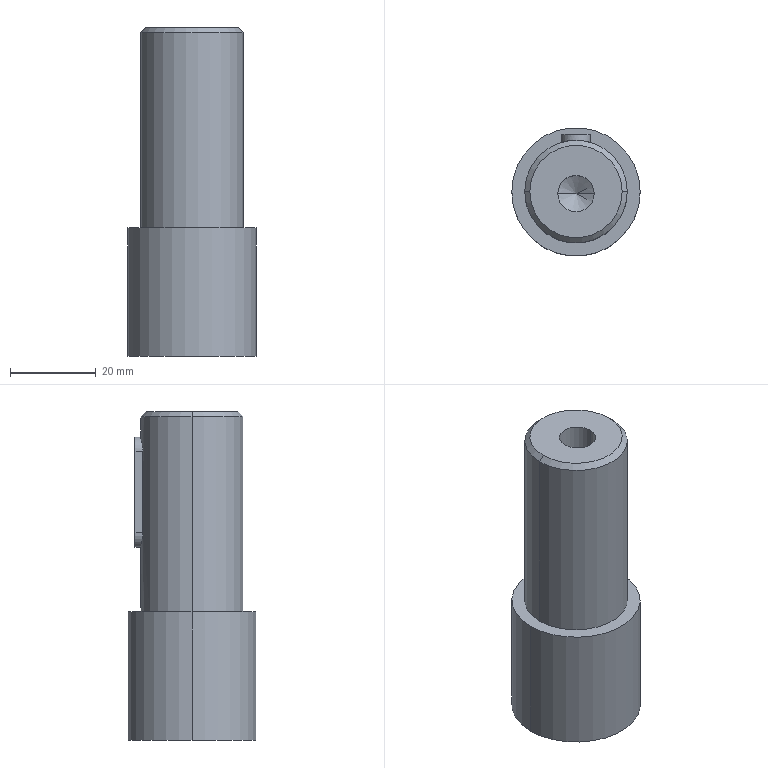Part | STEP file | XB output shaft_100_165_28.step | 1 solid | 24 faces | box 30 x 30 x 76.8 mm | volume 41146 mm3 | cylinder 9 | plane 8 | cone 7 | commonest cylinder face diameters 6.72 x3 8.5 x2 24 x2 30 x2
STEP:
#1=CARTESIAN_POINT('',(-4.25,0.,-98.603));
#2=VERTEX_POINT('',#1);
#3=CARTESIAN_POINT('',(4.25,0.,-98.603));
#4=VERTEX_POINT('',#3);
#5=CARTESIAN_POINT('',(0.,0.,-98.603));
#6=DIRECTION('',(0.,0.,1.));
#7=DIRECTION('',(1.,0.,0.));
#8=AXIS2_PLACEMENT_3D('',#5,#6,#7);
#9=CIRCLE('',#8,4.25);
#10=EDGE_CURVE('',#2,#4,#9,.T.);
#11=ORIENTED_EDGE('',*,*,#10,.F.);
#12=CARTESIAN_POINT('',(-4.25,0.,-74.103));
#13=VERTEX_POINT('',#12);
#14=CARTESIAN_POINT('',(-4.25,0.,-74.103));
#15=DIRECTION('',(0.,0.,1.));
#16=VECTOR('',#15,1000.);
#17=LINE('',#14,#16);
#18=EDGE_CURVE('',#2,#13,#17,.T.);
#19=ORIENTED_EDGE('',*,*,#18,.T.);
#20=CARTESIAN_POINT('',(4.25,0.,-74.103));
#21=VERTEX_POINT('',#20);
#22=CARTESIAN_POINT('',(0.,0.,-74.103));
#23=DIRECTION('',(0.,0.,1.));
#24=DIRECTION('',(1.,0.,0.));
#25=AXIS2_PLACEMENT_3D('',#22,#23,#24);
#26=CIRCLE('',#25,4.25);
#27=EDGE_CURVE('',#13,#21,#26,.T.);
#28=ORIENTED_EDGE('',*,*,#27,.T.);
#29=CARTESIAN_POINT('',(4.25,0.,-74.103));
#30=DIRECTION('',(0.,0.,1.));
#31=VECTOR('',#30,1000.);
#32=LINE('',#29,#31);
#33=EDGE_CURVE('',#4,#21,#32,.T.);
#34=ORIENTED_EDGE('',*,*,#33,.F.);
#35=EDGE_LOOP('',(#11,#19,#28,#34));
#36=FACE_OUTER_BOUND('',#35,.T.);
#37=CARTESIAN_POINT('',(0.,0.,-74.103));
#38=DIRECTION('',(0.,0.,1.));
#39=DIRECTION('',(1.,0.,0.));
#40=AXIS2_PLACEMENT_3D('',#37,#38,#39);
#41=CYLINDRICAL_SURFACE('',#40,4.25);
#42=ADVANCED_FACE('',(#36),#41,.F.);
#43=CARTESIAN_POINT('',(0.,0.,-101.156));
#44=VERTEX_POINT('',#43);
#45=CARTESIAN_POINT('',(4.25,0.,-98.603));
#46=DIRECTION('',(0.8572,0.,0.515));
#47=VECTOR('',#46,1000.);
#48=LINE('',#45,#47);
#49=EDGE_CURVE('',#44,#4,#48,.T.);
#50=ORIENTED_EDGE('',*,*,#49,.F.);
#51=CARTESIAN_POINT('',(-4.25,0.,-98.603));
#52=DIRECTION('',(-0.8572,0.,0.515));
#53=VECTOR('',#52,1000.);
#54=LINE('',#51,#53);
#55=EDGE_CURVE('',#44,#2,#54,.T.);
#56=ORIENTED_EDGE('',*,*,#55,.T.);
#57=ORIENTED_EDGE('',*,*,#10,.T.);
#58=EDGE_LOOP('',(#50,#56,#57));
#59=FACE_OUTER_BOUND('',#58,.T.);
#60=CARTESIAN_POINT('',(0.,0.,-98.603));
#61=DIRECTION('',(0.,0.,1.));
#62=DIRECTION('',(1.,0.,0.));
#63=AXIS2_PLACEMENT_3D('',#60,#61,#62);
#64=CONICAL_SURFACE('',#63,4.25,1.03);
#65=ADVANCED_FACE('',(#59),#64,.F.);
#66=CARTESIAN_POINT('',(-15.,0.4853,-150.903));
#67=VERTEX_POINT('',#66);
#68=CARTESIAN_POINT('',(15.,0.4853,-150.903));
#69=VERTEX_POINT('',#68);
#70=CARTESIAN_POINT('',(0.000002753,0.4853,-150.903));
#71=DIRECTION('',(0.,0.,-1.));
#72=DIRECTION('',(-1.,0.,0.));
#73=AXIS2_PLACEMENT_3D('',#70,#71,#72);
#74=CIRCLE('',#73,15.);
#75=EDGE_CURVE('',#67,#69,#74,.T.);
#76=ORIENTED_EDGE('',*,*,#75,.F.);
#77=CARTESIAN_POINT('',(-15.,0.4853,-120.903));
#78=VERTEX_POINT('',#77);
#79=CARTESIAN_POINT('',(-15.,0.4853,-150.903));
#80=DIRECTION('',(0.,0.,1.));
#81=VECTOR('',#80,1000.);
#82=LINE('',#79,#81);
#83=EDGE_CURVE('',#67,#78,#82,.T.);
#84=ORIENTED_EDGE('',*,*,#83,.T.);
#85=CARTESIAN_POINT('',(15.,0.4853,-120.903));
#86=VERTEX_POINT('',#85);
#87=CARTESIAN_POINT('',(0.000002753,0.4853,-120.903));
#88=DIRECTION('',(0.,0.,-1.));
#89=DIRECTION('',(-1.,0.,0.));
#90=AXIS2_PLACEMENT_3D('',#87,#88,#89);
#91=CIRCLE('',#90,15.);
#92=EDGE_CURVE('',#78,#86,#91,.T.);
#93=ORIENTED_EDGE('',*,*,#92,.T.);
#94=CARTESIAN_POINT('',(15.,0.4853,-150.903));
#95=DIRECTION('',(0.,0.,1.));
#96=VECTOR('',#95,1000.);
#97=LINE('',#94,#96);
#98=EDGE_CURVE('',#69,#86,#97,.T.);
#99=ORIENTED_EDGE('',*,*,#98,.F.);
#100=EDGE_LOOP('',(#76,#84,#93,#99));
#101=FACE_OUTER_BOUND('',#100,.T.);
#102=CARTESIAN_POINT('',(0.000002753,0.4853,-150.903));
#103=DIRECTION('',(0.,0.,1.));
#104=DIRECTION('',(1.,0.,0.));
#105=AXIS2_PLACEMENT_3D('',#102,#103,#104);
#106=CYLINDRICAL_SURFACE('',#105,15.);
#107=ADVANCED_FACE('',(#101),#106,.T.);
#108=CARTESIAN_POINT('',(-3.36,12.005,-83.403));
#109=VERTEX_POINT('',#108);
#110=CARTESIAN_POINT('',(-3.36,12.005,-102.423));
#111=VERTEX_POINT('',#110);
#112=CARTESIAN_POINT('',(-3.36,12.005,-74.103));
#113=DIRECTION('',(0.,0.,-1.));
#114=VECTOR('',#113,1000.);
#115=LINE('',#112,#114);
#116=EDGE_CURVE('',#109,#111,#115,.T.);
#117=ORIENTED_EDGE('',*,*,#116,.T.);
#118=CARTESIAN_POINT('',(0.000002753,12.485,-105.783));
#119=VERTEX_POINT('',#118);
#120=CARTESIAN_POINT('',(-3.36,12.005,-102.423));
#121=CARTESIAN_POINT('',(-3.36,12.005,-102.646));
#122=CARTESIAN_POINT('',(-3.338,12.012,-102.865));
#123=CARTESIAN_POINT('',(-3.252,12.036,-103.295));
#124=CARTESIAN_POINT('',(-3.187,12.055,-103.509));
#125=CARTESIAN_POINT('',(-3.018,12.1,-103.915));
#126=CARTESIAN_POINT('',(-2.915,12.127,-104.108));
#127=CARTESIAN_POINT('',(-2.672,12.185,-104.472));
#128=CARTESIAN_POINT('',(-2.531,12.216,-104.644));
#129=CARTESIAN_POINT('',(-2.223,12.279,-104.952));
#130=CARTESIAN_POINT('',(-2.054,12.31,-105.09));
#131=CARTESIAN_POINT('',(-1.688,12.367,-105.336));
#132=CARTESIAN_POINT('',(-1.494,12.394,-105.44));
#133=CARTESIAN_POINT('',(-1.091,12.437,-105.608));
#134=CARTESIAN_POINT('',(-0.8782,12.455,-105.673));
#135=CARTESIAN_POINT('',(-0.4433,12.479,-105.761));
#136=CARTESIAN_POINT('',(-0.223,12.485,-105.783));
#137=CARTESIAN_POINT('',(0.000002753,12.485,-105.783));
#138=B_SPLINE_CURVE_WITH_KNOTS('',3,(#120,#121,#122,#123,#124,#125,#126,#127,#128,#129,#130,#131,#132,#133,#134,#135,#136,#137),.UNSPECIFIED.,.F.,.F.,(4,2,2,2,2,2,2,2,4),(0.,0.0006594,0.001319,0.001978,0.002638,0.003297,0.003957,0.004616,0.005275),.UNSPECIFIED.);
#139=EDGE_CURVE('',#111,#119,#138,.T.);
#140=ORIENTED_EDGE('',*,*,#139,.T.);
#141=CARTESIAN_POINT('',(3.36,12.005,-102.423));
#142=VERTEX_POINT('',#141);
#143=CARTESIAN_POINT('',(0.000002753,12.485,-105.783));
#144=CARTESIAN_POINT('',(0.2231,12.485,-105.783));
#145=CARTESIAN_POINT('',(0.4422,12.479,-105.761));
#146=CARTESIAN_POINT('',(0.8729,12.455,-105.675));
#147=CARTESIAN_POINT('',(1.087,12.438,-105.609));
#148=CARTESIAN_POINT('',(1.493,12.394,-105.441));
#149=CARTESIAN_POINT('',(1.686,12.368,-105.337));
#150=CARTESIAN_POINT('',(2.05,12.31,-105.094));
#151=CARTESIAN_POINT('',(2.221,12.279,-104.953));
#152=CARTESIAN_POINT('',(2.53,12.217,-104.645));
#153=CARTESIAN_POINT('',(2.668,12.186,-104.477));
#154=CARTESIAN_POINT('',(2.914,12.127,-104.11));
#155=CARTESIAN_POINT('',(3.018,12.1,-103.916));
#156=CARTESIAN_POINT('',(3.186,12.055,-103.513));
#157=CARTESIAN_POINT('',(3.251,12.037,-103.301));
#158=CARTESIAN_POINT('',(3.338,12.012,-102.866));
#159=CARTESIAN_POINT('',(3.36,12.005,-102.646));
#160=CARTESIAN_POINT('',(3.36,12.005,-102.423));
#161=B_SPLINE_CURVE_WITH_KNOTS('',3,(#143,#144,#145,#146,#147,#148,#149,#150,#151,#152,#153,#154,#155,#156,#157,#158,#159,#160),.UNSPECIFIED.,.F.,.F.,(4,2,2,2,2,2,2,2,4),(0.005275,0.005935,0.006594,0.007254,0.007913,0.008573,0.009232,0.009891,0.01055),.UNSPECIFIED.);
#162=EDGE_CURVE('',#119,#142,#161,.T.);
#163=ORIENTED_EDGE('',*,*,#162,.T.);
#164=CARTESIAN_POINT('',(3.36,12.005,-83.403));
#165=VERTEX_POINT('',#164);
#166=CARTESIAN_POINT('',(3.36,12.005,-74.103));
#167=DIRECTION('',(0.,0.,1.));
#168=VECTOR('',#167,1000.);
#169=LINE('',#166,#168);
#170=EDGE_CURVE('',#142,#165,#169,.T.);
#171=ORIENTED_EDGE('',*,*,#170,.T.);
#172=CARTESIAN_POINT('',(3.36,12.005,-83.403));
#173=CARTESIAN_POINT('',(3.36,12.005,-83.179));
#174=CARTESIAN_POINT('',(3.338,12.012,-82.96));
#175=CARTESIAN_POINT('',(3.252,12.036,-82.529));
#176=CARTESIAN_POINT('',(3.187,12.055,-82.315));
#177=CARTESIAN_POINT('',(3.018,12.1,-81.909));
#178=CARTESIAN_POINT('',(2.915,12.127,-81.717));
#179=CARTESIAN_POINT('',(2.671,12.185,-81.352));
#180=CARTESIAN_POINT('',(2.53,12.217,-81.181));
#181=CARTESIAN_POINT('',(2.222,12.279,-80.873));
#182=CARTESIAN_POINT('',(2.054,12.31,-80.734));
#183=CARTESIAN_POINT('',(1.687,12.368,-80.488));
#184=CARTESIAN_POINT('',(1.493,12.394,-80.385));
#185=CARTESIAN_POINT('',(1.089,12.437,-80.216));
#186=CARTESIAN_POINT('',(0.8764,12.455,-80.151));
#187=CARTESIAN_POINT('',(0.4422,12.479,-80.064));
#188=CARTESIAN_POINT('',(0.2235,12.485,-80.043));
#189=CARTESIAN_POINT('',(-0.2172,12.485,-80.042));
#190=CARTESIAN_POINT('',(-0.441,12.479,-80.064));
#191=CARTESIAN_POINT('',(-0.8729,12.455,-80.15));
#192=CARTESIAN_POINT('',(-1.083,12.438,-80.214));
#193=CARTESIAN_POINT('',(-1.695,12.372,-80.468));
#194=CARTESIAN_POINT('',(-2.064,12.311,-80.715));
#195=CARTESIAN_POINT('',(-2.53,12.217,-81.181));
#196=CARTESIAN_POINT('',(-2.669,12.185,-81.349));
#197=CARTESIAN_POINT('',(-2.912,12.127,-81.712));
#198=CARTESIAN_POINT('',(-3.018,12.1,-81.909));
#199=CARTESIAN_POINT('',(-3.186,12.055,-82.314));
#200=CARTESIAN_POINT('',(-3.25,12.037,-82.523));
#201=CARTESIAN_POINT('',(-3.338,12.012,-82.956));
#202=CARTESIAN_POINT('',(-3.36,12.005,-83.179));
#203=CARTESIAN_POINT('',(-3.36,12.005,-83.403));
#204=B_SPLINE_CURVE_WITH_KNOTS('',3,(#172,#173,#174,#175,#176,#177,#178,#179,#180,#181,#182,#183,#184,#185,#186,#187,#188,#189,#190,#191,#192,#193,#194,#195,#196,#197,#198,#199,#200,#201,#202,#203),.UNSPECIFIED.,.F.,.F.,(4,2,2,2,2,2,2,2,2,2,2,2,2,2,2,4),(0.,0.0006596,0.001319,0.001979,0.002639,0.003298,0.003958,0.004618,0.005277,0.005937,0.006596,0.007916,0.008575,0.009235,0.009895,0.01055),.UNSPECIFIED.);
#205=EDGE_CURVE('',#165,#109,#204,.T.);
#206=ORIENTED_EDGE('',*,*,#205,.T.);
#207=EDGE_LOOP('',(#117,#140,#163,#171,#206));
#208=FACE_BOUND('',#207,.T.);
#209=CARTESIAN_POINT('',(12.,0.4853,-120.903));
#210=VERTEX_POINT('',#209);
#211=CARTESIAN_POINT('',(-12.,0.4853,-120.903));
#212=VERTEX_POINT('',#211);
#213=CARTESIAN_POINT('',(0.000002753,0.4853,-120.903));
#214=DIRECTION('',(0.,0.,1.));
#215=DIRECTION('',(-1.,0.,0.));
#216=AXIS2_PLACEMENT_3D('',#213,#214,#215);
#217=CIRCLE('',#216,12.);
#218=EDGE_CURVE('',#210,#212,#217,.T.);
#219=ORIENTED_EDGE('',*,*,#218,.T.);
#220=CARTESIAN_POINT('',(-12.,0.4853,-75.303));
#221=VERTEX_POINT('',#220);
#222=CARTESIAN_POINT('',(-12.,0.4853,-74.103));
#223=DIRECTION('',(0.,0.,1.));
#224=VECTOR('',#223,1000.);
#225=LINE('',#222,#224);
#226=EDGE_CURVE('',#212,#221,#225,.T.);
#227=ORIENTED_EDGE('',*,*,#226,.T.);
#228=CARTESIAN_POINT('',(12.,0.4853,-75.303));
#229=VERTEX_POINT('',#228);
#230=CARTESIAN_POINT('',(0.000002753,0.4853,-75.303));
#231=DIRECTION('',(0.,0.,-1.));
#232=DIRECTION('',(1.,0.,0.));
#233=AXIS2_PLACEMENT_3D('',#230,#231,#232);
#234=CIRCLE('',#233,12.);
#235=EDGE_CURVE('',#221,#229,#234,.T.);
#236=ORIENTED_EDGE('',*,*,#235,.T.);
#237=CARTESIAN_POINT('',(12.,0.4853,-74.103));
#238=DIRECTION('',(0.,0.,1.));
#239=VECTOR('',#238,1000.);
#240=LINE('',#237,#239);
#241=EDGE_CURVE('',#210,#229,#240,.T.);
#242=ORIENTED_EDGE('',*,*,#241,.F.);
#243=EDGE_LOOP('',(#219,#227,#236,#242));
#244=FACE_OUTER_BOUND('',#243,.T.);
#245=CARTESIAN_POINT('',(0.000002753,0.4853,-74.103));
#246=DIRECTION('',(0.,0.,1.));
#247=DIRECTION('',(1.,0.,0.));
#248=AXIS2_PLACEMENT_3D('',#245,#246,#247);
#249=CYLINDRICAL_SURFACE('',#248,12.);
#250=ADVANCED_FACE('',(#208,#244),#249,.T.);
#251=CARTESIAN_POINT('',(-10.8,0.4853,-74.103));
#252=VERTEX_POINT('',#251);
#253=CARTESIAN_POINT('',(10.8,0.4853,-74.103));
#254=VERTEX_POINT('',#253);
#255=CARTESIAN_POINT('',(0.000002753,0.4853,-74.103));
#256=DIRECTION('',(0.,0.,-1.));
#257=DIRECTION('',(-1.,0.,0.));
#258=AXIS2_PLACEMENT_3D('',#255,#256,#257);
#259=CIRCLE('',#258,10.8);
#260=EDGE_CURVE('',#252,#254,#259,.T.);
#261=ORIENTED_EDGE('',*,*,#260,.T.);
#262=CARTESIAN_POINT('',(12.,0.4853,-75.303));
#263=DIRECTION('',(0.7071,0.,-0.7071));
#264=VECTOR('',#263,1000.);
#265=LINE('',#262,#264);
#266=EDGE_CURVE('',#254,#229,#265,.T.);
#267=ORIENTED_EDGE('',*,*,#266,.T.);
#268=ORIENTED_EDGE('',*,*,#235,.F.);
#269=CARTESIAN_POINT('',(-12.,0.4853,-75.303));
#270=DIRECTION('',(-0.7071,0.,-0.7071));
#271=VECTOR('',#270,1000.);
#272=LINE('',#269,#271);
#273=EDGE_CURVE('',#252,#221,#272,.T.);
#274=ORIENTED_EDGE('',*,*,#273,.F.);
#275=EDGE_LOOP('',(#261,#267,#268,#274));
#276=FACE_OUTER_BOUND('',#275,.T.);
#277=CARTESIAN_POINT('',(0.000002753,0.4853,-75.303));
#278=DIRECTION('',(0.,0.,-1.));
#279=DIRECTION('',(-1.,0.,0.));
#280=AXIS2_PLACEMENT_3D('',#277,#278,#279);
#281=CONICAL_SURFACE('',#280,12.,0.7854);
#282=ADVANCED_FACE('',(#276),#281,.T.);
#283=CARTESIAN_POINT('',(-3.36,13.805,-102.423));
#284=VERTEX_POINT('',#283);
#285=CARTESIAN_POINT('',(0.000002753,13.805,-105.783));
#286=VERTEX_POINT('',#285);
#287=CARTESIAN_POINT('',(0.000002753,13.805,-102.423));
#288=DIRECTION('',(0.,-1.,0.));
#289=DIRECTION('',(0.,0.,-1.));
#290=AXIS2_PLACEMENT_3D('',#287,#288,#289);
#291=CIRCLE('',#290,3.36);
#292=EDGE_CURVE('',#284,#286,#291,.T.);
#293=ORIENTED_EDGE('',*,*,#292,.T.);
#294=CARTESIAN_POINT('',(0.000002753,13.925,-105.783));
#295=DIRECTION('',(0.,-1.,0.));
#296=VECTOR('',#295,1000.);
#297=LINE('',#294,#296);
#298=EDGE_CURVE('',#286,#119,#297,.T.);
#299=ORIENTED_EDGE('',*,*,#298,.T.);
#300=ORIENTED_EDGE('',*,*,#139,.F.);
#301=CARTESIAN_POINT('',(-3.36,13.925,-102.423));
#302=DIRECTION('',(0.,1.,0.));
#303=VECTOR('',#302,1000.);
#304=LINE('',#301,#303);
#305=EDGE_CURVE('',#111,#284,#304,.T.);
#306=ORIENTED_EDGE('',*,*,#305,.T.);
#307=EDGE_LOOP('',(#293,#299,#300,#306));
#308=FACE_OUTER_BOUND('',#307,.T.);
#309=CARTESIAN_POINT('',(0.000002753,13.925,-102.423));
#310=DIRECTION('',(0.,-1.,0.));
#311=DIRECTION('',(0.,0.,-1.));
#312=AXIS2_PLACEMENT_3D('',#309,#310,#311);
#313=CYLINDRICAL_SURFACE('',#312,3.36);
#314=ADVANCED_FACE('',(#308),#313,.T.);
#315=CARTESIAN_POINT('',(-3.24,13.925,-102.423));
#316=VERTEX_POINT('',#315);
#317=CARTESIAN_POINT('',(0.000002753,13.925,-105.663));
#318=VERTEX_POINT('',#317);
#319=CARTESIAN_POINT('',(0.000002753,13.925,-102.423));
#320=DIRECTION('',(0.,-1.,0.));
#321=DIRECTION('',(0.,0.,-1.));
#322=AXIS2_PLACEMENT_3D('',#319,#320,#321);
#323=CIRCLE('',#322,3.24);
#324=EDGE_CURVE('',#316,#318,#323,.T.);
#325=ORIENTED_EDGE('',*,*,#324,.T.);
#326=CARTESIAN_POINT('',(0.000002753,13.805,-105.783));
#327=DIRECTION('',(0.,-0.7071,-0.7071));
#328=VECTOR('',#327,1000.);
#329=LINE('',#326,#328);
#330=EDGE_CURVE('',#318,#286,#329,.T.);
#331=ORIENTED_EDGE('',*,*,#330,.T.);
#332=ORIENTED_EDGE('',*,*,#292,.F.);
#333=CARTESIAN_POINT('',(-3.24,13.925,-102.423));
#334=DIRECTION('',(0.7071,0.7071,0.));
#335=VECTOR('',#334,1000.);
#336=LINE('',#333,#335);
#337=EDGE_CURVE('',#284,#316,#336,.T.);
#338=ORIENTED_EDGE('',*,*,#337,.T.);
#339=EDGE_LOOP('',(#325,#331,#332,#338));
#340=FACE_OUTER_BOUND('',#339,.T.);
#341=CARTESIAN_POINT('',(0.000002753,13.805,-102.423));
#342=DIRECTION('',(0.,-1.,0.));
#343=DIRECTION('',(0.,0.,-1.));
#344=AXIS2_PLACEMENT_3D('',#341,#342,#343);
#345=CONICAL_SURFACE('',#344,3.36,0.7854);
#346=ADVANCED_FACE('',(#340),#345,.T.);
#347=ORIENTED_EDGE('',*,*,#226,.F.);
#348=CARTESIAN_POINT('',(0.000002753,0.4853,-120.903));
#349=DIRECTION('',(0.,0.,1.));
#350=DIRECTION('',(-1.,0.,0.));
#351=AXIS2_PLACEMENT_3D('',#348,#349,#350);
#352=CIRCLE('',#351,12.);
#353=EDGE_CURVE('',#212,#210,#352,.T.);
#354=ORIENTED_EDGE('',*,*,#353,.T.);
#355=ORIENTED_EDGE('',*,*,#241,.T.);
#356=CARTESIAN_POINT('',(0.000002753,0.4853,-75.303));
#357=DIRECTION('',(0.,0.,-1.));
#358=DIRECTION('',(1.,0.,0.));
#359=AXIS2_PLACEMENT_3D('',#356,#357,#358);
#360=CIRCLE('',#359,12.);
#361=EDGE_CURVE('',#229,#221,#360,.T.);
#362=ORIENTED_EDGE('',*,*,#361,.T.);
#363=EDGE_LOOP('',(#347,#354,#355,#362));
#364=FACE_OUTER_BOUND('',#363,.T.);
#365=CARTESIAN_POINT('',(0.000002753,0.4853,-74.103));
#366=DIRECTION('',(0.,0.,1.));
#367=DIRECTION('',(1.,0.,0.));
#368=AXIS2_PLACEMENT_3D('',#365,#366,#367);
#369=CYLINDRICAL_SURFACE('',#368,12.);
#370=ADVANCED_FACE('',(#364),#369,.T.);
#371=ORIENTED_EDGE('',*,*,#266,.F.);
#372=CARTESIAN_POINT('',(0.000002753,0.4853,-74.103));
#373=DIRECTION('',(0.,0.,-1.));
#374=DIRECTION('',(-1.,0.,0.));
#375=AXIS2_PLACEMENT_3D('',#372,#373,#374);
#376=CIRCLE('',#375,10.8);
#377=EDGE_CURVE('',#254,#252,#376,.T.);
#378=ORIENTED_EDGE('',*,*,#377,.T.);
#379=ORIENTED_EDGE('',*,*,#273,.T.);
#380=ORIENTED_EDGE('',*,*,#361,.F.);
#381=EDGE_LOOP('',(#371,#378,#379,#380));
#382=FACE_OUTER_BOUND('',#381,.T.);
#383=CARTESIAN_POINT('',(0.000002753,0.4853,-75.303));
#384=DIRECTION('',(0.,0.,-1.));
#385=DIRECTION('',(-1.,0.,0.));
#386=AXIS2_PLACEMENT_3D('',#383,#384,#385);
#387=CONICAL_SURFACE('',#386,12.,0.7854);
#388=ADVANCED_FACE('',(#382),#387,.T.);
#389=CARTESIAN_POINT('',(0.,0.,-74.103));
#390=DIRECTION('',(0.,0.,1.));
#391=DIRECTION('',(1.,0.,0.));
#392=AXIS2_PLACEMENT_3D('',#389,#390,#391);
#393=CIRCLE('',#392,4.25);
#394=EDGE_CURVE('',#21,#13,#393,.T.);
#395=ORIENTED_EDGE('',*,*,#394,.F.);
#396=ORIENTED_EDGE('',*,*,#27,.F.);
#397=EDGE_LOOP('',(#395,#396));
#398=FACE_BOUND('',#397,.T.);
#399=ORIENTED_EDGE('',*,*,#260,.F.);
#400=ORIENTED_EDGE('',*,*,#377,.F.);
#401=EDGE_LOOP('',(#399,#400));
#402=FACE_OUTER_BOUND('',#401,.T.);
#403=CARTESIAN_POINT('',(0.000002753,11.285,-74.103));
#404=DIRECTION('',(0.,0.,-1.));
#405=DIRECTION('',(-1.,0.,0.));
#406=AXIS2_PLACEMENT_3D('',#403,#404,#405);
#407=PLANE('',#406);
#408=ADVANCED_FACE('',(#398,#402),#407,.F.);
#409=ORIENTED_EDGE('',*,*,#298,.F.);
#410=CARTESIAN_POINT('',(3.36,13.805,-102.423));
#411=VERTEX_POINT('',#410);
#412=CARTESIAN_POINT('',(0.000002753,13.805,-102.423));
#413=DIRECTION('',(0.,-1.,0.));
#414=DIRECTION('',(0.,0.,-1.));
#415=AXIS2_PLACEMENT_3D('',#412,#413,#414);
#416=CIRCLE('',#415,3.36);
#417=EDGE_CURVE('',#286,#411,#416,.T.);
#418=ORIENTED_EDGE('',*,*,#417,.T.);
#419=CARTESIAN_POINT('',(3.36,13.925,-102.423));
#420=DIRECTION('',(0.,-1.,0.));
#421=VECTOR('',#420,1000.);
#422=LINE('',#419,#421);
#423=EDGE_CURVE('',#411,#142,#422,.T.);
#424=ORIENTED_EDGE('',*,*,#423,.T.);
#425=ORIENTED_EDGE('',*,*,#162,.F.);
#426=EDGE_LOOP('',(#409,#418,#424,#425));
#427=FACE_OUTER_BOUND('',#426,.T.);
#428=CARTESIAN_POINT('',(0.000002753,13.925,-102.423));
#429=DIRECTION('',(0.,-1.,0.));
#430=DIRECTION('',(0.,0.,-1.));
#431=AXIS2_PLACEMENT_3D('',#428,#429,#430);
#432=CYLINDRICAL_SURFACE('',#431,3.36);
#433=ADVANCED_FACE('',(#427),#432,.T.);
#434=CARTESIAN_POINT('',(-3.36,13.805,-83.403));
#435=VERTEX_POINT('',#434);
#436=CARTESIAN_POINT('',(-3.36,13.805,-102.423));
#437=DIRECTION('',(0.,0.,1.));
#438=VECTOR('',#437,1000.);
#439=LINE('',#436,#438);
#440=EDGE_CURVE('',#284,#435,#439,.T.);
#441=ORIENTED_EDGE('',*,*,#440,.F.);
#442=ORIENTED_EDGE('',*,*,#305,.F.);
#443=ORIENTED_EDGE('',*,*,#116,.F.);
#444=CARTESIAN_POINT('',(-3.36,13.925,-83.403));
#445=DIRECTION('',(0.,-1.,0.));
#446=VECTOR('',#445,1000.);
#447=LINE('',#444,#446);
#448=EDGE_CURVE('',#435,#109,#447,.T.);
#449=ORIENTED_EDGE('',*,*,#448,.F.);
#450=EDGE_LOOP('',(#441,#442,#443,#449));
#451=FACE_OUTER_BOUND('',#450,.T.);
#452=CARTESIAN_POINT('',(-3.36,13.925,-102.423));
#453=DIRECTION('',(1.,0.,0.));
#454=DIRECTION('',(0.,0.,-1.));
#455=AXIS2_PLACEMENT_3D('',#452,#453,#454);
#456=PLANE('',#455);
#457=ADVANCED_FACE('',(#451),#456,.F.);
#458=ORIENTED_EDGE('',*,*,#448,.T.);
#459=ORIENTED_EDGE('',*,*,#205,.F.);
#460=CARTESIAN_POINT('',(3.36,13.805,-83.403));
#461=VERTEX_POINT('',#460);
#462=CARTESIAN_POINT('',(3.36,13.925,-83.403));
#463=DIRECTION('',(0.,1.,0.));
#464=VECTOR('',#463,1000.);
#465=LINE('',#462,#464);
#466=EDGE_CURVE('',#165,#461,#465,.T.);
#467=ORIENTED_EDGE('',*,*,#466,.T.);
#468=CARTESIAN_POINT('',(0.000002753,13.805,-83.403));
#469=DIRECTION('',(0.,-1.,0.));
#470=DIRECTION('',(0.,0.,-1.));
#471=AXIS2_PLACEMENT_3D('',#468,#469,#470);
#472=CIRCLE('',#471,3.36);
#473=EDGE_CURVE('',#461,#435,#472,.T.);
#474=ORIENTED_EDGE('',*,*,#473,.T.);
#475=EDGE_LOOP('',(#458,#459,#467,#474));
#476=FACE_OUTER_BOUND('',#475,.T.);
#477=CARTESIAN_POINT('',(0.000002753,13.925,-83.403));
#478=DIRECTION('',(0.,-1.,0.));
#479=DIRECTION('',(0.,0.,-1.));
#480=AXIS2_PLACEMENT_3D('',#477,#478,#479);
#481=CYLINDRICAL_SURFACE('',#480,3.36);
#482=ADVANCED_FACE('',(#476),#481,.T.);
#483=CARTESIAN_POINT('',(3.36,13.805,-102.423));
#484=DIRECTION('',(0.,0.,-1.));
#485=VECTOR('',#484,1000.);
#486=LINE('',#483,#485);
#487=EDGE_CURVE('',#461,#411,#486,.T.);
#488=ORIENTED_EDGE('',*,*,#487,.F.);
#489=ORIENTED_EDGE('',*,*,#466,.F.);
#490=ORIENTED_EDGE('',*,*,#170,.F.);
#491=ORIENTED_EDGE('',*,*,#423,.F.);
#492=EDGE_LOOP('',(#488,#489,#490,#491));
#493=FACE_OUTER_BOUND('',#492,.T.);
#494=CARTESIAN_POINT('',(3.36,13.925,-102.423));
#495=DIRECTION('',(-1.,0.,0.));
#496=DIRECTION('',(0.,0.,1.));
#497=AXIS2_PLACEMENT_3D('',#494,#495,#496);
#498=PLANE('',#497);
#499=ADVANCED_FACE('',(#493),#498,.F.);
#500=ORIENTED_EDGE('',*,*,#330,.F.);
#501=CARTESIAN_POINT('',(3.24,13.925,-102.423));
#502=VERTEX_POINT('',#501);
#503=CARTESIAN_POINT('',(0.000002753,13.925,-102.423));
#504=DIRECTION('',(0.,-1.,0.));
#505=DIRECTION('',(0.,0.,-1.));
#506=AXIS2_PLACEMENT_3D('',#503,#504,#505);
#507=CIRCLE('',#506,3.24);
#508=EDGE_CURVE('',#318,#502,#507,.T.);
#509=ORIENTED_EDGE('',*,*,#508,.T.);
#510=CARTESIAN_POINT('',(3.24,13.925,-102.423));
#511=DIRECTION('',(-0.7071,0.7071,0.));
#512=VECTOR('',#511,1000.);
#513=LINE('',#510,#512);
#514=EDGE_CURVE('',#411,#502,#513,.T.);
#515=ORIENTED_EDGE('',*,*,#514,.F.);
#516=ORIENTED_EDGE('',*,*,#417,.F.);
#517=EDGE_LOOP('',(#500,#509,#515,#516));
#518=FACE_OUTER_BOUND('',#517,.T.);
#519=CARTESIAN_POINT('',(0.000002753,13.805,-102.423));
#520=DIRECTION('',(0.,-1.,0.));
#521=DIRECTION('',(0.,0.,-1.));
#522=AXIS2_PLACEMENT_3D('',#519,#520,#521);
#523=CONICAL_SURFACE('',#522,3.36,0.7854);
#524=ADVANCED_FACE('',(#518),#523,.T.);
#525=CARTESIAN_POINT('',(-3.24,13.925,-83.403));
#526=VERTEX_POINT('',#525);
#527=CARTESIAN_POINT('',(-3.24,13.925,-83.403));
#528=DIRECTION('',(0.7071,0.7071,0.));
#529=VECTOR('',#528,1000.);
#530=LINE('',#527,#529);
#531=EDGE_CURVE('',#435,#526,#530,.T.);
#532=ORIENTED_EDGE('',*,*,#531,.T.);
#533=CARTESIAN_POINT('',(-3.24,13.925,-102.423));
#534=DIRECTION('',(0.,0.,-1.));
#535=VECTOR('',#534,1000.);
#536=LINE('',#533,#535);
#537=EDGE_CURVE('',#526,#316,#536,.T.);
#538=ORIENTED_EDGE('',*,*,#537,.T.);
#539=ORIENTED_EDGE('',*,*,#337,.F.);
#540=ORIENTED_EDGE('',*,*,#440,.T.);
#541=EDGE_LOOP('',(#532,#538,#539,#540));
#542=FACE_OUTER_BOUND('',#541,.T.);
#543=CARTESIAN_POINT('',(-3.24,13.925,-102.423));
#544=DIRECTION('',(-0.7071,0.7071,0.));
#545=DIRECTION('',(-0.7071,-0.7071,0.));
#546=AXIS2_PLACEMENT_3D('',#543,#544,#545);
#547=PLANE('',#546);
#548=ADVANCED_FACE('',(#542),#547,.T.);
#549=CARTESIAN_POINT('',(3.24,13.925,-83.403));
#550=VERTEX_POINT('',#549);
#551=CARTESIAN_POINT('',(3.24,13.925,-83.403));
#552=DIRECTION('',(-0.7071,0.7071,0.));
#553=VECTOR('',#552,1000.);
#554=LINE('',#551,#553);
#555=EDGE_CURVE('',#461,#550,#554,.T.);
#556=ORIENTED_EDGE('',*,*,#555,.T.);
#557=CARTESIAN_POINT('',(0.000002753,13.925,-83.403));
#558=DIRECTION('',(0.,-1.,0.));
#559=DIRECTION('',(0.,0.,-1.));
#560=AXIS2_PLACEMENT_3D('',#557,#558,#559);
#561=CIRCLE('',#560,3.24);
#562=EDGE_CURVE('',#550,#526,#561,.T.);
#563=ORIENTED_EDGE('',*,*,#562,.T.);
#564=ORIENTED_EDGE('',*,*,#531,.F.);
#565=ORIENTED_EDGE('',*,*,#473,.F.);
#566=EDGE_LOOP('',(#556,#563,#564,#565));
#567=FACE_OUTER_BOUND('',#566,.T.);
#568=CARTESIAN_POINT('',(0.000002753,13.805,-83.403));
#569=DIRECTION('',(0.,-1.,0.));
#570=DIRECTION('',(0.,0.,-1.));
#571=AXIS2_PLACEMENT_3D('',#568,#569,#570);
#572=CONICAL_SURFACE('',#571,3.36,0.7854);
#573=ADVANCED_FACE('',(#567),#572,.T.);
#574=ORIENTED_EDGE('',*,*,#514,.T.);
#575=CARTESIAN_POINT('',(3.24,13.925,-102.423));
#576=DIRECTION('',(0.,0.,1.));
#577=VECTOR('',#576,1000.);
#578=LINE('',#575,#577);
#579=EDGE_CURVE('',#502,#550,#578,.T.);
#580=ORIENTED_EDGE('',*,*,#579,.T.);
#581=ORIENTED_EDGE('',*,*,#555,.F.);
#582=ORIENTED_EDGE('',*,*,#487,.T.);
#583=EDGE_LOOP('',(#574,#580,#581,#582));
#584=FACE_OUTER_BOUND('',#583,.T.);
#585=CARTESIAN_POINT('',(3.24,13.925,-102.423));
#586=DIRECTION('',(0.7071,0.7071,0.));
#587=DIRECTION('',(-0.7071,0.7071,0.));
#588=AXIS2_PLACEMENT_3D('',#585,#586,#587);
#589=PLANE('',#588);
#590=ADVANCED_FACE('',(#584),#589,.T.);
#591=ORIENTED_EDGE('',*,*,#324,.F.);
#592=ORIENTED_EDGE('',*,*,#537,.F.);
#593=ORIENTED_EDGE('',*,*,#562,.F.);
#594=ORIENTED_EDGE('',*,*,#579,.F.);
#595=ORIENTED_EDGE('',*,*,#508,.F.);
#596=EDGE_LOOP('',(#591,#592,#593,#594,#595));
#597=FACE_OUTER_BOUND('',#596,.T.);
#598=CARTESIAN_POINT('',(0.000002753,13.925,-102.423));
#599=DIRECTION('',(0.,1.,0.));
#600=DIRECTION('',(0.,0.,1.));
#601=AXIS2_PLACEMENT_3D('',#598,#599,#600);
#602=PLANE('',#601);
#603=ADVANCED_FACE('',(#597),#602,.T.);
#604=ORIENTED_EDGE('',*,*,#83,.F.);
#605=CARTESIAN_POINT('',(0.000002753,0.4853,-150.903));
#606=DIRECTION('',(0.,0.,-1.));
#607=DIRECTION('',(-1.,0.,0.));
#608=AXIS2_PLACEMENT_3D('',#605,#606,#607);
#609=CIRCLE('',#608,15.);
#610=EDGE_CURVE('',#69,#67,#609,.T.);
#611=ORIENTED_EDGE('',*,*,#610,.F.);
#612=ORIENTED_EDGE('',*,*,#98,.T.);
#613=CARTESIAN_POINT('',(0.000002753,0.4853,-120.903));
#614=DIRECTION('',(0.,0.,-1.));
#615=DIRECTION('',(-1.,0.,0.));
#616=AXIS2_PLACEMENT_3D('',#613,#614,#615);
#617=CIRCLE('',#616,15.);
#618=EDGE_CURVE('',#86,#78,#617,.T.);
#619=ORIENTED_EDGE('',*,*,#618,.T.);
#620=EDGE_LOOP('',(#604,#611,#612,#619));
#621=FACE_OUTER_BOUND('',#620,.T.);
#622=CARTESIAN_POINT('',(0.000002753,0.4853,-150.903));
#623=DIRECTION('',(0.,0.,1.));
#624=DIRECTION('',(1.,0.,0.));
#625=AXIS2_PLACEMENT_3D('',#622,#623,#624);
#626=CYLINDRICAL_SURFACE('',#625,15.);
#627=ADVANCED_FACE('',(#621),#626,.T.);
#628=ORIENTED_EDGE('',*,*,#610,.T.);
#629=ORIENTED_EDGE('',*,*,#75,.T.);
#630=EDGE_LOOP('',(#628,#629));
#631=FACE_OUTER_BOUND('',#630,.T.);
#632=CARTESIAN_POINT('',(0.000002753,0.4853,-150.903));
#633=DIRECTION('',(0.,0.,-1.));
#634=DIRECTION('',(-1.,0.,0.));
#635=AXIS2_PLACEMENT_3D('',#632,#633,#634);
#636=PLANE('',#635);
#637=ADVANCED_FACE('',(#631),#636,.T.);
#638=ORIENTED_EDGE('',*,*,#218,.F.);
#639=ORIENTED_EDGE('',*,*,#353,.F.);
#640=EDGE_LOOP('',(#638,#639));
#641=FACE_BOUND('',#640,.T.);
#642=ORIENTED_EDGE('',*,*,#618,.F.);
#643=ORIENTED_EDGE('',*,*,#92,.F.);
#644=EDGE_LOOP('',(#642,#643));
#645=FACE_OUTER_BOUND('',#644,.T.);
#646=CARTESIAN_POINT('',(0.000002753,0.4853,-120.903));
#647=DIRECTION('',(0.,0.,-1.));
#648=DIRECTION('',(-1.,0.,0.));
#649=AXIS2_PLACEMENT_3D('',#646,#647,#648);
#650=PLANE('',#649);
#651=ADVANCED_FACE('',(#641,#645),#650,.F.);
#652=ORIENTED_EDGE('',*,*,#55,.F.);
#653=ORIENTED_EDGE('',*,*,#49,.T.);
#654=CARTESIAN_POINT('',(0.,0.,-98.603));
#655=DIRECTION('',(0.,0.,1.));
#656=DIRECTION('',(1.,0.,0.));
#657=AXIS2_PLACEMENT_3D('',#654,#655,#656);
#658=CIRCLE('',#657,4.25);
#659=EDGE_CURVE('',#4,#2,#658,.T.);
#660=ORIENTED_EDGE('',*,*,#659,.T.);
#661=EDGE_LOOP('',(#652,#653,#660));
#662=FACE_OUTER_BOUND('',#661,.T.);
#663=CARTESIAN_POINT('',(0.,0.,-98.603));
#664=DIRECTION('',(0.,0.,1.));
#665=DIRECTION('',(1.,0.,0.));
#666=AXIS2_PLACEMENT_3D('',#663,#664,#665);
#667=CONICAL_SURFACE('',#666,4.25,1.03);
#668=ADVANCED_FACE('',(#662),#667,.F.);
#669=ORIENTED_EDGE('',*,*,#18,.F.);
#670=ORIENTED_EDGE('',*,*,#659,.F.);
#671=ORIENTED_EDGE('',*,*,#33,.T.);
#672=ORIENTED_EDGE('',*,*,#394,.T.);
#673=EDGE_LOOP('',(#669,#670,#671,#672));
#674=FACE_OUTER_BOUND('',#673,.T.);
#675=CARTESIAN_POINT('',(0.,0.,-74.103));
#676=DIRECTION('',(0.,0.,1.));
#677=DIRECTION('',(1.,0.,0.));
#678=AXIS2_PLACEMENT_3D('',#675,#676,#677);
#679=CYLINDRICAL_SURFACE('',#678,4.25);
#680=ADVANCED_FACE('',(#674),#679,.F.);
#681=CLOSED_SHELL('',(#42,#65,#107,#250,#282,#314,#346,#370,#388,#408,#433,#457,#482,#499,#524,#548,#573,#590,#603,#627,#637,#651,#668,#680));
#682=MANIFOLD_SOLID_BREP('',#681);
#683=CARTESIAN_POINT('',(0.,0.,0.));
#684=DIRECTION('',(0.,0.,1.));
#685=DIRECTION('',(1.,0.,0.));
#686=AXIS2_PLACEMENT_3D('',#683,#684,#685);
#687=(LENGTH_UNIT()NAMED_UNIT(*)SI_UNIT(.MILLI.,.METRE.));
#688=UNCERTAINTY_MEASURE_WITH_UNIT(LENGTH_MEASURE(0.00001),#687,'','');
#689=(NAMED_UNIT(*)PLANE_ANGLE_UNIT()SI_UNIT($,.RADIAN.));
#690=(NAMED_UNIT(*)SI_UNIT($,.STERADIAN.)SOLID_ANGLE_UNIT());
#691=(GEOMETRIC_REPRESENTATION_CONTEXT(3)GLOBAL_UNCERTAINTY_ASSIGNED_CONTEXT((#688))GLOBAL_UNIT_ASSIGNED_CONTEXT((#687,#689,#690))REPRESENTATION_CONTEXT('',''));
#692=ADVANCED_BREP_SHAPE_REPRESENTATION('',(#682,#686),#691);